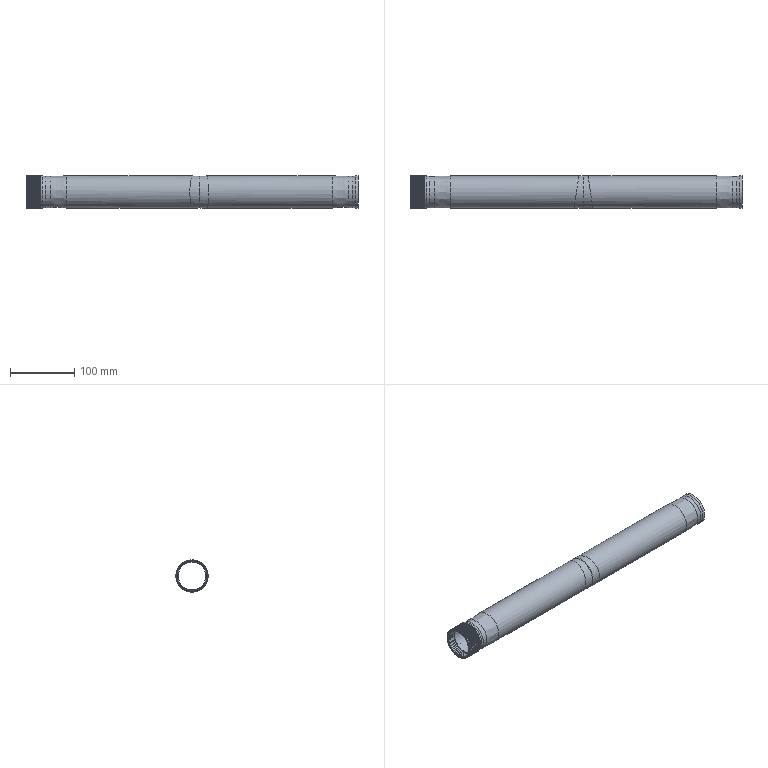Part | STEP file | 610B0701 | 1 solid | 2822 faces | box 515 x 50 x 50 mm | volume 253052 mm3 | plane 1606 | cylinder 1212 | cone 4 | commonest cylinder face diameters 0.82 x1200 50 x7 44 x2 48.5 x2 43 x1